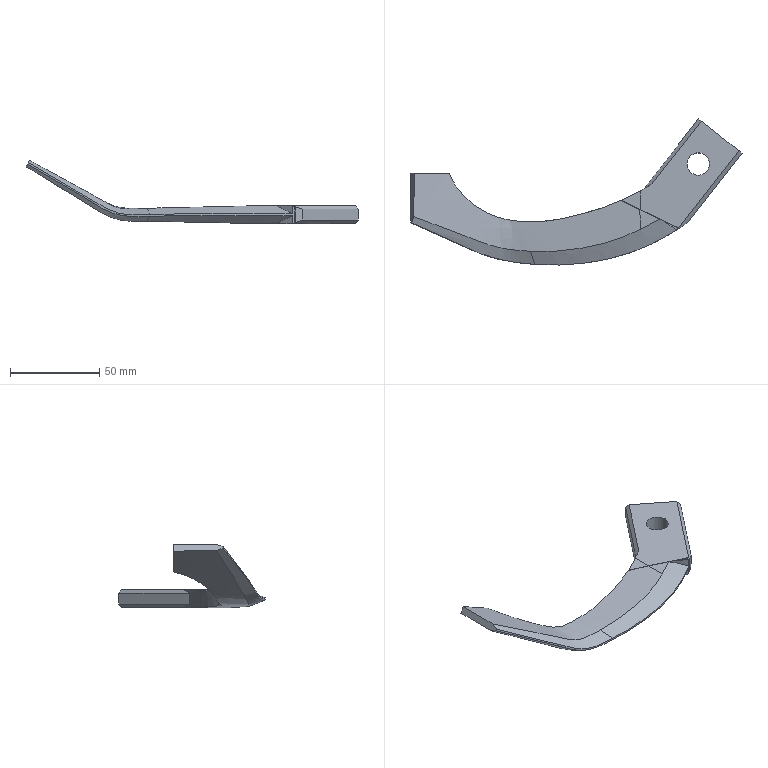Part | SolidWorks | features ICE 2, Chamfer 1, CombineBodies 1, Deform 1, DeleteBody 1, Extrusion 1, FillRefSurface 1, MirrorPattern 1, RefCurve 1, Split 1, SurfCut 1, SweepCut 1 | 2 solids | 37 faces | box 186.248 x 81.99 x 35.546 mm | volume 40697 mm3 | spline 20 | plane 13 | cylinder 4 | commonest cylinder face diameters 12.5 x2 243.979 x1 299.971 x1